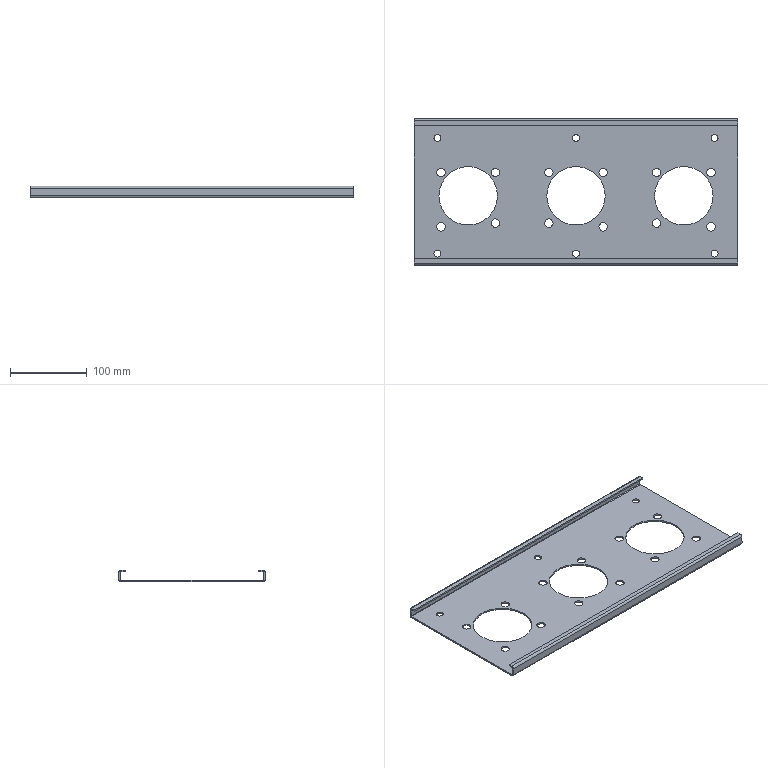Part | SolidWorks | features EdgeFlange 4, FlatPattern 1, SMBaseFlange 1, SheetMetal 1 | 1 solid | 80 faces | box 420 x 190 x 15 mm | volume 158753 mm3 | cylinder 50 | plane 30 | commonest cylinder face diameters 11 x24 9 x12 76 x6 1.473 x4 5.473 x4